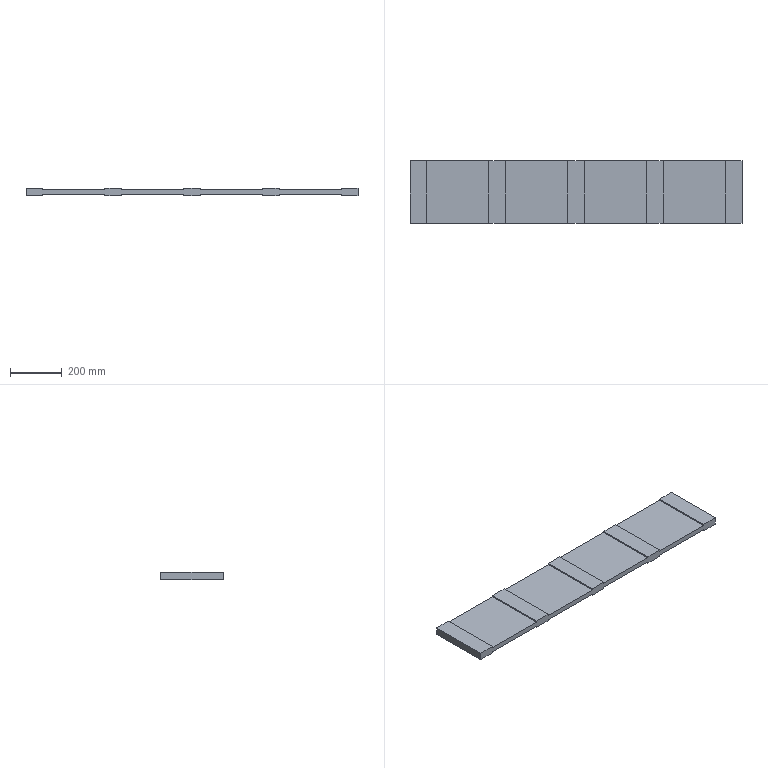Part | SolidWorks | features Extrusion 1, ICE 1 | 1 solid | 38 faces | box 1280 x 240 x 30 mm | volume 6912000 mm3 | plane 38
STEP:
#1=CARTESIAN_POINT('',(672.,0.,20.));
#2=VERTEX_POINT('',#1);
#3=CARTESIAN_POINT('',(912.,0.,20.));
#4=VERTEX_POINT('',#3);
#5=CARTESIAN_POINT('',(0.,0.,20.));
#6=DIRECTION('',(1.,0.,0.));
#7=VECTOR('',#6,1000.);
#8=LINE('',#5,#7);
#9=EDGE_CURVE('',#2,#4,#8,.T.);
#10=ORIENTED_EDGE('',*,*,#9,.T.);
#11=CARTESIAN_POINT('',(912.,240.,20.));
#12=VERTEX_POINT('',#11);
#13=CARTESIAN_POINT('',(912.,0.,20.));
#14=DIRECTION('',(0.,1.,0.));
#15=VECTOR('',#14,1000.);
#16=LINE('',#13,#15);
#17=EDGE_CURVE('',#4,#12,#16,.T.);
#18=ORIENTED_EDGE('',*,*,#17,.T.);
#19=CARTESIAN_POINT('',(672.,240.,20.));
#20=VERTEX_POINT('',#19);
#21=CARTESIAN_POINT('',(0.,240.,20.));
#22=DIRECTION('',(-1.,0.,0.));
#23=VECTOR('',#22,1000.);
#24=LINE('',#21,#23);
#25=EDGE_CURVE('',#12,#20,#24,.T.);
#26=ORIENTED_EDGE('',*,*,#25,.T.);
#27=CARTESIAN_POINT('',(672.,0.,20.));
#28=DIRECTION('',(0.,-1.,0.));
#29=VECTOR('',#28,1000.);
#30=LINE('',#27,#29);
#31=EDGE_CURVE('',#20,#2,#30,.T.);
#32=ORIENTED_EDGE('',*,*,#31,.T.);
#33=EDGE_LOOP('',(#10,#18,#26,#32));
#34=FACE_OUTER_BOUND('',#33,.T.);
#35=CARTESIAN_POINT('',(0.,0.,20.));
#36=DIRECTION('',(0.,0.,-1.));
#37=DIRECTION('',(-1.,0.,0.));
#38=AXIS2_PLACEMENT_3D('',#35,#36,#37);
#39=PLANE('',#38);
#40=ADVANCED_FACE('',(#34),#39,.F.);
#41=CARTESIAN_POINT('',(912.,0.,0.));
#42=VERTEX_POINT('',#41);
#43=CARTESIAN_POINT('',(912.,240.,0.));
#44=VERTEX_POINT('',#43);
#45=CARTESIAN_POINT('',(912.,0.,0.));
#46=DIRECTION('',(0.,1.,0.));
#47=VECTOR('',#46,1000.);
#48=LINE('',#45,#47);
#49=EDGE_CURVE('',#42,#44,#48,.T.);
#50=ORIENTED_EDGE('',*,*,#49,.F.);
#51=CARTESIAN_POINT('',(672.,0.,0.));
#52=VERTEX_POINT('',#51);
#53=CARTESIAN_POINT('',(0.,0.,0.));
#54=DIRECTION('',(1.,0.,0.));
#55=VECTOR('',#54,1000.);
#56=LINE('',#53,#55);
#57=EDGE_CURVE('',#52,#42,#56,.T.);
#58=ORIENTED_EDGE('',*,*,#57,.F.);
#59=CARTESIAN_POINT('',(672.,240.,0.));
#60=VERTEX_POINT('',#59);
#61=CARTESIAN_POINT('',(672.,0.,0.));
#62=DIRECTION('',(0.,-1.,0.));
#63=VECTOR('',#62,1000.);
#64=LINE('',#61,#63);
#65=EDGE_CURVE('',#60,#52,#64,.T.);
#66=ORIENTED_EDGE('',*,*,#65,.F.);
#67=CARTESIAN_POINT('',(0.,240.,0.));
#68=DIRECTION('',(-1.,0.,0.));
#69=VECTOR('',#68,1000.);
#70=LINE('',#67,#69);
#71=EDGE_CURVE('',#44,#60,#70,.T.);
#72=ORIENTED_EDGE('',*,*,#71,.F.);
#73=EDGE_LOOP('',(#50,#58,#66,#72));
#74=FACE_OUTER_BOUND('',#73,.T.);
#75=CARTESIAN_POINT('',(0.,0.,0.));
#76=DIRECTION('',(0.,0.,-1.));
#77=DIRECTION('',(-1.,0.,0.));
#78=AXIS2_PLACEMENT_3D('',#75,#76,#77);
#79=PLANE('',#78);
#80=ADVANCED_FACE('',(#74),#79,.T.);
#81=CARTESIAN_POINT('',(368.,0.,20.));
#82=VERTEX_POINT('',#81);
#83=CARTESIAN_POINT('',(608.,0.,20.));
#84=VERTEX_POINT('',#83);
#85=CARTESIAN_POINT('',(0.,0.,20.));
#86=DIRECTION('',(1.,0.,0.));
#87=VECTOR('',#86,1000.);
#88=LINE('',#85,#87);
#89=EDGE_CURVE('',#82,#84,#88,.T.);
#90=ORIENTED_EDGE('',*,*,#89,.T.);
#91=CARTESIAN_POINT('',(608.,240.,20.));
#92=VERTEX_POINT('',#91);
#93=CARTESIAN_POINT('',(608.,0.,20.));
#94=DIRECTION('',(0.,1.,0.));
#95=VECTOR('',#94,1000.);
#96=LINE('',#93,#95);
#97=EDGE_CURVE('',#84,#92,#96,.T.);
#98=ORIENTED_EDGE('',*,*,#97,.T.);
#99=CARTESIAN_POINT('',(368.,240.,20.));
#100=VERTEX_POINT('',#99);
#101=CARTESIAN_POINT('',(0.,240.,20.));
#102=DIRECTION('',(-1.,0.,0.));
#103=VECTOR('',#102,1000.);
#104=LINE('',#101,#103);
#105=EDGE_CURVE('',#92,#100,#104,.T.);
#106=ORIENTED_EDGE('',*,*,#105,.T.);
#107=CARTESIAN_POINT('',(368.,0.,20.));
#108=DIRECTION('',(0.,-1.,0.));
#109=VECTOR('',#108,1000.);
#110=LINE('',#107,#109);
#111=EDGE_CURVE('',#100,#82,#110,.T.);
#112=ORIENTED_EDGE('',*,*,#111,.T.);
#113=EDGE_LOOP('',(#90,#98,#106,#112));
#114=FACE_OUTER_BOUND('',#113,.T.);
#115=CARTESIAN_POINT('',(0.,0.,20.));
#116=DIRECTION('',(0.,0.,-1.));
#117=DIRECTION('',(-1.,0.,0.));
#118=AXIS2_PLACEMENT_3D('',#115,#116,#117);
#119=PLANE('',#118);
#120=ADVANCED_FACE('',(#114),#119,.F.);
#121=CARTESIAN_POINT('',(608.,0.,0.));
#122=VERTEX_POINT('',#121);
#123=CARTESIAN_POINT('',(608.,240.,0.));
#124=VERTEX_POINT('',#123);
#125=CARTESIAN_POINT('',(608.,0.,0.));
#126=DIRECTION('',(0.,1.,0.));
#127=VECTOR('',#126,1000.);
#128=LINE('',#125,#127);
#129=EDGE_CURVE('',#122,#124,#128,.T.);
#130=ORIENTED_EDGE('',*,*,#129,.F.);
#131=CARTESIAN_POINT('',(368.,0.,0.));
#132=VERTEX_POINT('',#131);
#133=CARTESIAN_POINT('',(0.,0.,0.));
#134=DIRECTION('',(1.,0.,0.));
#135=VECTOR('',#134,1000.);
#136=LINE('',#133,#135);
#137=EDGE_CURVE('',#132,#122,#136,.T.);
#138=ORIENTED_EDGE('',*,*,#137,.F.);
#139=CARTESIAN_POINT('',(368.,240.,0.));
#140=VERTEX_POINT('',#139);
#141=CARTESIAN_POINT('',(368.,0.,0.));
#142=DIRECTION('',(0.,-1.,0.));
#143=VECTOR('',#142,1000.);
#144=LINE('',#141,#143);
#145=EDGE_CURVE('',#140,#132,#144,.T.);
#146=ORIENTED_EDGE('',*,*,#145,.F.);
#147=CARTESIAN_POINT('',(0.,240.,0.));
#148=DIRECTION('',(-1.,0.,0.));
#149=VECTOR('',#148,1000.);
#150=LINE('',#147,#149);
#151=EDGE_CURVE('',#124,#140,#150,.T.);
#152=ORIENTED_EDGE('',*,*,#151,.F.);
#153=EDGE_LOOP('',(#130,#138,#146,#152));
#154=FACE_OUTER_BOUND('',#153,.T.);
#155=CARTESIAN_POINT('',(0.,0.,0.));
#156=DIRECTION('',(0.,0.,-1.));
#157=DIRECTION('',(-1.,0.,0.));
#158=AXIS2_PLACEMENT_3D('',#155,#156,#157);
#159=PLANE('',#158);
#160=ADVANCED_FACE('',(#154),#159,.T.);
#161=CARTESIAN_POINT('',(64.,0.,20.));
#162=VERTEX_POINT('',#161);
#163=CARTESIAN_POINT('',(304.,0.,20.));
#164=VERTEX_POINT('',#163);
#165=CARTESIAN_POINT('',(0.,0.,20.));
#166=DIRECTION('',(1.,0.,0.));
#167=VECTOR('',#166,1000.);
#168=LINE('',#165,#167);
#169=EDGE_CURVE('',#162,#164,#168,.T.);
#170=ORIENTED_EDGE('',*,*,#169,.T.);
#171=CARTESIAN_POINT('',(304.,240.,20.));
#172=VERTEX_POINT('',#171);
#173=CARTESIAN_POINT('',(304.,0.,20.));
#174=DIRECTION('',(0.,1.,0.));
#175=VECTOR('',#174,1000.);
#176=LINE('',#173,#175);
#177=EDGE_CURVE('',#164,#172,#176,.T.);
#178=ORIENTED_EDGE('',*,*,#177,.T.);
#179=CARTESIAN_POINT('',(64.,240.,20.));
#180=VERTEX_POINT('',#179);
#181=CARTESIAN_POINT('',(0.,240.,20.));
#182=DIRECTION('',(-1.,0.,0.));
#183=VECTOR('',#182,1000.);
#184=LINE('',#181,#183);
#185=EDGE_CURVE('',#172,#180,#184,.T.);
#186=ORIENTED_EDGE('',*,*,#185,.T.);
#187=CARTESIAN_POINT('',(64.,0.,20.));
#188=DIRECTION('',(0.,-1.,0.));
#189=VECTOR('',#188,1000.);
#190=LINE('',#187,#189);
#191=EDGE_CURVE('',#180,#162,#190,.T.);
#192=ORIENTED_EDGE('',*,*,#191,.T.);
#193=EDGE_LOOP('',(#170,#178,#186,#192));
#194=FACE_OUTER_BOUND('',#193,.T.);
#195=CARTESIAN_POINT('',(0.,0.,20.));
#196=DIRECTION('',(0.,0.,-1.));
#197=DIRECTION('',(-1.,0.,0.));
#198=AXIS2_PLACEMENT_3D('',#195,#196,#197);
#199=PLANE('',#198);
#200=ADVANCED_FACE('',(#194),#199,.F.);
#201=CARTESIAN_POINT('',(304.,0.,0.));
#202=VERTEX_POINT('',#201);
#203=CARTESIAN_POINT('',(304.,240.,0.));
#204=VERTEX_POINT('',#203);
#205=CARTESIAN_POINT('',(304.,0.,0.));
#206=DIRECTION('',(0.,1.,0.));
#207=VECTOR('',#206,1000.);
#208=LINE('',#205,#207);
#209=EDGE_CURVE('',#202,#204,#208,.T.);
#210=ORIENTED_EDGE('',*,*,#209,.F.);
#211=CARTESIAN_POINT('',(64.,0.,0.));
#212=VERTEX_POINT('',#211);
#213=CARTESIAN_POINT('',(0.,0.,0.));
#214=DIRECTION('',(1.,0.,0.));
#215=VECTOR('',#214,1000.);
#216=LINE('',#213,#215);
#217=EDGE_CURVE('',#212,#202,#216,.T.);
#218=ORIENTED_EDGE('',*,*,#217,.F.);
#219=CARTESIAN_POINT('',(64.,240.,0.));
#220=VERTEX_POINT('',#219);
#221=CARTESIAN_POINT('',(64.,0.,0.));
#222=DIRECTION('',(0.,-1.,0.));
#223=VECTOR('',#222,1000.);
#224=LINE('',#221,#223);
#225=EDGE_CURVE('',#220,#212,#224,.T.);
#226=ORIENTED_EDGE('',*,*,#225,.F.);
#227=CARTESIAN_POINT('',(0.,240.,0.));
#228=DIRECTION('',(-1.,0.,0.));
#229=VECTOR('',#228,1000.);
#230=LINE('',#227,#229);
#231=EDGE_CURVE('',#204,#220,#230,.T.);
#232=ORIENTED_EDGE('',*,*,#231,.F.);
#233=EDGE_LOOP('',(#210,#218,#226,#232));
#234=FACE_OUTER_BOUND('',#233,.T.);
#235=CARTESIAN_POINT('',(0.,0.,0.));
#236=DIRECTION('',(0.,0.,-1.));
#237=DIRECTION('',(-1.,0.,0.));
#238=AXIS2_PLACEMENT_3D('',#235,#236,#237);
#239=PLANE('',#238);
#240=ADVANCED_FACE('',(#234),#239,.T.);
#241=CARTESIAN_POINT('',(0.,240.,25.));
#242=VERTEX_POINT('',#241);
#243=CARTESIAN_POINT('',(0.,240.,-5.));
#244=VERTEX_POINT('',#243);
#245=CARTESIAN_POINT('',(0.,240.,20.));
#246=DIRECTION('',(0.,0.,-1.));
#247=VECTOR('',#246,1000.);
#248=LINE('',#245,#247);
#249=EDGE_CURVE('',#242,#244,#248,.T.);
#250=ORIENTED_EDGE('',*,*,#249,.T.);
#251=CARTESIAN_POINT('',(0.,0.,-5.));
#252=VERTEX_POINT('',#251);
#253=CARTESIAN_POINT('',(0.,240.,-5.));
#254=DIRECTION('',(0.,-1.,0.));
#255=VECTOR('',#254,1000.);
#256=LINE('',#253,#255);
#257=EDGE_CURVE('',#244,#252,#256,.T.);
#258=ORIENTED_EDGE('',*,*,#257,.T.);
#259=CARTESIAN_POINT('',(0.,0.,25.));
#260=VERTEX_POINT('',#259);
#261=CARTESIAN_POINT('',(0.,0.,20.));
#262=DIRECTION('',(0.,0.,-1.));
#263=VECTOR('',#262,1000.);
#264=LINE('',#261,#263);
#265=EDGE_CURVE('',#260,#252,#264,.T.);
#266=ORIENTED_EDGE('',*,*,#265,.F.);
#267=CARTESIAN_POINT('',(0.,240.,25.));
#268=DIRECTION('',(0.,-1.,0.));
#269=VECTOR('',#268,1000.);
#270=LINE('',#267,#269);
#271=EDGE_CURVE('',#242,#260,#270,.T.);
#272=ORIENTED_EDGE('',*,*,#271,.F.);
#273=EDGE_LOOP('',(#250,#258,#266,#272));
#274=FACE_OUTER_BOUND('',#273,.T.);
#275=CARTESIAN_POINT('',(0.,0.,20.));
#276=DIRECTION('',(1.,0.,0.));
#277=DIRECTION('',(0.,0.,-1.));
#278=AXIS2_PLACEMENT_3D('',#275,#276,#277);
#279=PLANE('',#278);
#280=ADVANCED_FACE('',(#274),#279,.F.);
#281=CARTESIAN_POINT('',(976.,0.,0.));
#282=VERTEX_POINT('',#281);
#283=CARTESIAN_POINT('',(1216.,0.,0.));
#284=VERTEX_POINT('',#283);
#285=CARTESIAN_POINT('',(0.,0.,0.));
#286=DIRECTION('',(1.,0.,0.));
#287=VECTOR('',#286,1000.);
#288=LINE('',#285,#287);
#289=EDGE_CURVE('',#282,#284,#288,.T.);
#290=ORIENTED_EDGE('',*,*,#289,.T.);
#291=CARTESIAN_POINT('',(1216.,0.,-5.));
#292=VERTEX_POINT('',#291);
#293=CARTESIAN_POINT('',(1216.,0.,25.));
#294=DIRECTION('',(0.,0.,-1.));
#295=VECTOR('',#294,1000.);
#296=LINE('',#293,#295);
#297=EDGE_CURVE('',#284,#292,#296,.T.);
#298=ORIENTED_EDGE('',*,*,#297,.T.);
#299=CARTESIAN_POINT('',(1280.,0.,-5.));
#300=VERTEX_POINT('',#299);
#301=CARTESIAN_POINT('',(1216.,0.,-5.));
#302=DIRECTION('',(1.,0.,0.));
#303=VECTOR('',#302,1000.);
#304=LINE('',#301,#303);
#305=EDGE_CURVE('',#292,#300,#304,.T.);
#306=ORIENTED_EDGE('',*,*,#305,.T.);
#307=CARTESIAN_POINT('',(1280.,0.,25.));
#308=VERTEX_POINT('',#307);
#309=CARTESIAN_POINT('',(1280.,0.,25.));
#310=DIRECTION('',(0.,0.,1.));
#311=VECTOR('',#310,1000.);
#312=LINE('',#309,#311);
#313=EDGE_CURVE('',#300,#308,#312,.T.);
#314=ORIENTED_EDGE('',*,*,#313,.T.);
#315=CARTESIAN_POINT('',(1216.,0.,25.));
#316=VERTEX_POINT('',#315);
#317=CARTESIAN_POINT('',(1216.,0.,25.));
#318=DIRECTION('',(-1.,0.,0.));
#319=VECTOR('',#318,1000.);
#320=LINE('',#317,#319);
#321=EDGE_CURVE('',#308,#316,#320,.T.);
#322=ORIENTED_EDGE('',*,*,#321,.T.);
#323=CARTESIAN_POINT('',(1216.,0.,20.));
#324=VERTEX_POINT('',#323);
#325=CARTESIAN_POINT('',(1216.,0.,25.));
#326=DIRECTION('',(0.,0.,-1.));
#327=VECTOR('',#326,1000.);
#328=LINE('',#325,#327);
#329=EDGE_CURVE('',#316,#324,#328,.T.);
#330=ORIENTED_EDGE('',*,*,#329,.T.);
#331=CARTESIAN_POINT('',(976.,0.,20.));
#332=VERTEX_POINT('',#331);
#333=CARTESIAN_POINT('',(0.,0.,20.));
#334=DIRECTION('',(1.,0.,0.));
#335=VECTOR('',#334,1000.);
#336=LINE('',#333,#335);
#337=EDGE_CURVE('',#332,#324,#336,.T.);
#338=ORIENTED_EDGE('',*,*,#337,.F.);
#339=CARTESIAN_POINT('',(976.,0.,25.));
#340=VERTEX_POINT('',#339);
#341=CARTESIAN_POINT('',(976.,0.,25.));
#342=DIRECTION('',(0.,0.,1.));
#343=VECTOR('',#342,1000.);
#344=LINE('',#341,#343);
#345=EDGE_CURVE('',#332,#340,#344,.T.);
#346=ORIENTED_EDGE('',*,*,#345,.T.);
#347=CARTESIAN_POINT('',(912.,0.,25.));
#348=VERTEX_POINT('',#347);
#349=CARTESIAN_POINT('',(912.,0.,25.));
#350=DIRECTION('',(-1.,0.,0.));
#351=VECTOR('',#350,1000.);
#352=LINE('',#349,#351);
#353=EDGE_CURVE('',#340,#348,#352,.T.);
#354=ORIENTED_EDGE('',*,*,#353,.T.);
#355=CARTESIAN_POINT('',(912.,0.,25.));
#356=DIRECTION('',(0.,0.,-1.));
#357=VECTOR('',#356,1000.);
#358=LINE('',#355,#357);
#359=EDGE_CURVE('',#348,#4,#358,.T.);
#360=ORIENTED_EDGE('',*,*,#359,.T.);
#361=ORIENTED_EDGE('',*,*,#9,.F.);
#362=CARTESIAN_POINT('',(672.,0.,25.));
#363=VERTEX_POINT('',#362);
#364=CARTESIAN_POINT('',(672.,0.,25.));
#365=DIRECTION('',(0.,0.,1.));
#366=VECTOR('',#365,1000.);
#367=LINE('',#364,#366);
#368=EDGE_CURVE('',#2,#363,#367,.T.);
#369=ORIENTED_EDGE('',*,*,#368,.T.);
#370=CARTESIAN_POINT('',(608.,0.,25.));
#371=VERTEX_POINT('',#370);
#372=CARTESIAN_POINT('',(608.,0.,25.));
#373=DIRECTION('',(-1.,0.,0.));
#374=VECTOR('',#373,1000.);
#375=LINE('',#372,#374);
#376=EDGE_CURVE('',#363,#371,#375,.T.);
#377=ORIENTED_EDGE('',*,*,#376,.T.);
#378=CARTESIAN_POINT('',(608.,0.,25.));
#379=DIRECTION('',(0.,0.,-1.));
#380=VECTOR('',#379,1000.);
#381=LINE('',#378,#380);
#382=EDGE_CURVE('',#371,#84,#381,.T.);
#383=ORIENTED_EDGE('',*,*,#382,.T.);
#384=ORIENTED_EDGE('',*,*,#89,.F.);
#385=CARTESIAN_POINT('',(368.,0.,25.));
#386=VERTEX_POINT('',#385);
#387=CARTESIAN_POINT('',(368.,0.,25.));
#388=DIRECTION('',(0.,0.,1.));
#389=VECTOR('',#388,1000.);
#390=LINE('',#387,#389);
#391=EDGE_CURVE('',#82,#386,#390,.T.);
#392=ORIENTED_EDGE('',*,*,#391,.T.);
#393=CARTESIAN_POINT('',(304.,0.,25.));
#394=VERTEX_POINT('',#393);
#395=CARTESIAN_POINT('',(304.,0.,25.));
#396=DIRECTION('',(-1.,0.,0.));
#397=VECTOR('',#396,1000.);
#398=LINE('',#395,#397);
#399=EDGE_CURVE('',#386,#394,#398,.T.);
#400=ORIENTED_EDGE('',*,*,#399,.T.);
#401=CARTESIAN_POINT('',(304.,0.,25.));
#402=DIRECTION('',(0.,0.,-1.));
#403=VECTOR('',#402,1000.);
#404=LINE('',#401,#403);
#405=EDGE_CURVE('',#394,#164,#404,.T.);
#406=ORIENTED_EDGE('',*,*,#405,.T.);
#407=ORIENTED_EDGE('',*,*,#169,.F.);
#408=CARTESIAN_POINT('',(64.,0.,25.));
#409=VERTEX_POINT('',#408);
#410=CARTESIAN_POINT('',(64.,0.,-5.));
#411=DIRECTION('',(0.,0.,1.));
#412=VECTOR('',#411,1000.);
#413=LINE('',#410,#412);
#414=EDGE_CURVE('',#162,#409,#413,.T.);
#415=ORIENTED_EDGE('',*,*,#414,.T.);
#416=CARTESIAN_POINT('',(0.,0.,25.));
#417=DIRECTION('',(-1.,0.,0.));
#418=VECTOR('',#417,1000.);
#419=LINE('',#416,#418);
#420=EDGE_CURVE('',#409,#260,#419,.T.);
#421=ORIENTED_EDGE('',*,*,#420,.T.);
#422=ORIENTED_EDGE('',*,*,#265,.T.);
#423=CARTESIAN_POINT('',(64.,0.,-5.));
#424=VERTEX_POINT('',#423);
#425=CARTESIAN_POINT('',(0.,0.,-5.));
#426=DIRECTION('',(1.,0.,0.));
#427=VECTOR('',#426,1000.);
#428=LINE('',#425,#427);
#429=EDGE_CURVE('',#252,#424,#428,.T.);
#430=ORIENTED_EDGE('',*,*,#429,.T.);
#431=CARTESIAN_POINT('',(64.,0.,-5.));
#432=DIRECTION('',(0.,0.,1.));
#433=VECTOR('',#432,1000.);
#434=LINE('',#431,#433);
#435=EDGE_CURVE('',#424,#212,#434,.T.);
#436=ORIENTED_EDGE('',*,*,#435,.T.);
#437=ORIENTED_EDGE('',*,*,#217,.T.);
#438=CARTESIAN_POINT('',(304.,0.,-5.));
#439=VERTEX_POINT('',#438);
#440=CARTESIAN_POINT('',(304.,0.,25.));
#441=DIRECTION('',(0.,0.,-1.));
#442=VECTOR('',#441,1000.);
#443=LINE('',#440,#442);
#444=EDGE_CURVE('',#202,#439,#443,.T.);
#445=ORIENTED_EDGE('',*,*,#444,.T.);
#446=CARTESIAN_POINT('',(368.,0.,-5.));
#447=VERTEX_POINT('',#446);
#448=CARTESIAN_POINT('',(304.,0.,-5.));
#449=DIRECTION('',(1.,0.,0.));
#450=VECTOR('',#449,1000.);
#451=LINE('',#448,#450);
#452=EDGE_CURVE('',#439,#447,#451,.T.);
#453=ORIENTED_EDGE('',*,*,#452,.T.);
#454=CARTESIAN_POINT('',(368.,0.,25.));
#455=DIRECTION('',(0.,0.,1.));
#456=VECTOR('',#455,1000.);
#457=LINE('',#454,#456);
#458=EDGE_CURVE('',#447,#132,#457,.T.);
#459=ORIENTED_EDGE('',*,*,#458,.T.);
#460=ORIENTED_EDGE('',*,*,#137,.T.);
#461=CARTESIAN_POINT('',(608.,0.,-5.));
#462=VERTEX_POINT('',#461);
#463=CARTESIAN_POINT('',(608.,0.,25.));
#464=DIRECTION('',(0.,0.,-1.));
#465=VECTOR('',#464,1000.);
#466=LINE('',#463,#465);
#467=EDGE_CURVE('',#122,#462,#466,.T.);
#468=ORIENTED_EDGE('',*,*,#467,.T.);
#469=CARTESIAN_POINT('',(672.,0.,-5.));
#470=VERTEX_POINT('',#469);
#471=CARTESIAN_POINT('',(608.,0.,-5.));
#472=DIRECTION('',(1.,0.,0.));
#473=VECTOR('',#472,1000.);
#474=LINE('',#471,#473);
#475=EDGE_CURVE('',#462,#470,#474,.T.);
#476=ORIENTED_EDGE('',*,*,#475,.T.);
#477=CARTESIAN_POINT('',(672.,0.,25.));
#478=DIRECTION('',(0.,0.,1.));
#479=VECTOR('',#478,1000.);
#480=LINE('',#477,#479);
#481=EDGE_CURVE('',#470,#52,#480,.T.);
#482=ORIENTED_EDGE('',*,*,#481,.T.);
#483=ORIENTED_EDGE('',*,*,#57,.T.);
#484=CARTESIAN_POINT('',(912.,0.,-5.));
#485=VERTEX_POINT('',#484);
#486=CARTESIAN_POINT('',(912.,0.,25.));
#487=DIRECTION('',(0.,0.,-1.));
#488=VECTOR('',#487,1000.);
#489=LINE('',#486,#488);
#490=EDGE_CURVE('',#42,#485,#489,.T.);
#491=ORIENTED_EDGE('',*,*,#490,.T.);
#492=CARTESIAN_POINT('',(976.,0.,-5.));
#493=VERTEX_POINT('',#492);
#494=CARTESIAN_POINT('',(912.,0.,-5.));
#495=DIRECTION('',(1.,0.,0.));
#496=VECTOR('',#495,1000.);
#497=LINE('',#494,#496);
#498=EDGE_CURVE('',#485,#493,#497,.T.);
#499=ORIENTED_EDGE('',*,*,#498,.T.);
#500=CARTESIAN_POINT('',(976.,0.,25.));
#501=DIRECTION('',(0.,0.,1.));
#502=VECTOR('',#501,1000.);
#503=LINE('',#500,#502);
#504=EDGE_CURVE('',#493,#282,#503,.T.);
#505=ORIENTED_EDGE('',*,*,#504,.T.);
#506=EDGE_LOOP('',(#290,#298,#306,#314,#322,#330,#338,#346,#354,#360,#361,#369,#377,#383,#384,#392,#400,#406,#407,#415,#421,#422,#430,#436,#437,#445,#453,#459,#460,#468,#476,#482,#483,#491,#499,#505));
#507=FACE_OUTER_BOUND('',#506,.T.);
#508=CARTESIAN_POINT('',(0.,0.,20.));
#509=DIRECTION('',(0.,1.,0.));
#510=DIRECTION('',(0.,0.,1.));
#511=AXIS2_PLACEMENT_3D('',#508,#509,#510);
#512=PLANE('',#511);
#513=ADVANCED_FACE('',(#507),#512,.F.);
#514=CARTESIAN_POINT('',(1216.,240.,20.));
#515=VERTEX_POINT('',#514);
#516=CARTESIAN_POINT('',(976.,240.,20.));
#517=VERTEX_POINT('',#516);
#518=CARTESIAN_POINT('',(0.,240.,20.));
#519=DIRECTION('',(-1.,0.,0.));
#520=VECTOR('',#519,1000.);
#521=LINE('',#518,#520);
#522=EDGE_CURVE('',#515,#517,#521,.T.);
#523=ORIENTED_EDGE('',*,*,#522,.F.);
#524=CARTESIAN_POINT('',(1216.,240.,25.));
#525=VERTEX_POINT('',#524);
#526=CARTESIAN_POINT('',(1216.,240.,25.));
#527=DIRECTION('',(0.,0.,-1.));
#528=VECTOR('',#527,1000.);
#529=LINE('',#526,#528);
#530=EDGE_CURVE('',#525,#515,#529,.T.);
#531=ORIENTED_EDGE('',*,*,#530,.F.);
#532=CARTESIAN_POINT('',(1280.,240.,25.));
#533=VERTEX_POINT('',#532);
#534=CARTESIAN_POINT('',(1216.,240.,25.));
#535=DIRECTION('',(-1.,0.,0.));
#536=VECTOR('',#535,1000.);
#537=LINE('',#534,#536);
#538=EDGE_CURVE('',#533,#525,#537,.T.);
#539=ORIENTED_EDGE('',*,*,#538,.F.);
#540=CARTESIAN_POINT('',(1280.,240.,-5.));
#541=VERTEX_POINT('',#540);
#542=CARTESIAN_POINT('',(1280.,240.,25.));
#543=DIRECTION('',(0.,0.,1.));
#544=VECTOR('',#543,1000.);
#545=LINE('',#542,#544);
#546=EDGE_CURVE('',#541,#533,#545,.T.);
#547=ORIENTED_EDGE('',*,*,#546,.F.);
#548=CARTESIAN_POINT('',(1216.,240.,-5.));
#549=VERTEX_POINT('',#548);
#550=CARTESIAN_POINT('',(1216.,240.,-5.));
#551=DIRECTION('',(1.,0.,0.));
#552=VECTOR('',#551,1000.);
#553=LINE('',#550,#552);
#554=EDGE_CURVE('',#549,#541,#553,.T.);
#555=ORIENTED_EDGE('',*,*,#554,.F.);
#556=CARTESIAN_POINT('',(1216.,240.,0.));
#557=VERTEX_POINT('',#556);
#558=CARTESIAN_POINT('',(1216.,240.,25.));
#559=DIRECTION('',(0.,0.,-1.));
#560=VECTOR('',#559,1000.);
#561=LINE('',#558,#560);
#562=EDGE_CURVE('',#557,#549,#561,.T.);
#563=ORIENTED_EDGE('',*,*,#562,.F.);
#564=CARTESIAN_POINT('',(976.,240.,0.));
#565=VERTEX_POINT('',#564);
#566=CARTESIAN_POINT('',(0.,240.,0.));
#567=DIRECTION('',(-1.,0.,0.));
#568=VECTOR('',#567,1000.);
#569=LINE('',#566,#568);
#570=EDGE_CURVE('',#557,#565,#569,.T.);
#571=ORIENTED_EDGE('',*,*,#570,.T.);
#572=CARTESIAN_POINT('',(976.,240.,-5.));
#573=VERTEX_POINT('',#572);
#574=CARTESIAN_POINT('',(976.,240.,25.));
#575=DIRECTION('',(0.,0.,1.));
#576=VECTOR('',#575,1000.);
#577=LINE('',#574,#576);
#578=EDGE_CURVE('',#573,#565,#577,.T.);
#579=ORIENTED_EDGE('',*,*,#578,.F.);
#580=CARTESIAN_POINT('',(912.,240.,-5.));
#581=VERTEX_POINT('',#580);
#582=CARTESIAN_POINT('',(912.,240.,-5.));
#583=DIRECTION('',(1.,0.,0.));
#584=VECTOR('',#583,1000.);
#585=LINE('',#582,#584);
#586=EDGE_CURVE('',#581,#573,#585,.T.);
#587=ORIENTED_EDGE('',*,*,#586,.F.);
#588=CARTESIAN_POINT('',(912.,240.,25.));
#589=DIRECTION('',(0.,0.,-1.));
#590=VECTOR('',#589,1000.);
#591=LINE('',#588,#590);
#592=EDGE_CURVE('',#44,#581,#591,.T.);
#593=ORIENTED_EDGE('',*,*,#592,.F.);
#594=ORIENTED_EDGE('',*,*,#71,.T.);
#595=CARTESIAN_POINT('',(672.,240.,-5.));
#596=VERTEX_POINT('',#595);
#597=CARTESIAN_POINT('',(672.,240.,25.));
#598=DIRECTION('',(0.,0.,1.));
#599=VECTOR('',#598,1000.);
#600=LINE('',#597,#599);
#601=EDGE_CURVE('',#596,#60,#600,.T.);
#602=ORIENTED_EDGE('',*,*,#601,.F.);
#603=CARTESIAN_POINT('',(608.,240.,-5.));
#604=VERTEX_POINT('',#603);
#605=CARTESIAN_POINT('',(608.,240.,-5.));
#606=DIRECTION('',(1.,0.,0.));
#607=VECTOR('',#606,1000.);
#608=LINE('',#605,#607);
#609=EDGE_CURVE('',#604,#596,#608,.T.);
#610=ORIENTED_EDGE('',*,*,#609,.F.);
#611=CARTESIAN_POINT('',(608.,240.,25.));
#612=DIRECTION('',(0.,0.,-1.));
#613=VECTOR('',#612,1000.);
#614=LINE('',#611,#613);
#615=EDGE_CURVE('',#124,#604,#614,.T.);
#616=ORIENTED_EDGE('',*,*,#615,.F.);
#617=ORIENTED_EDGE('',*,*,#151,.T.);
#618=CARTESIAN_POINT('',(368.,240.,-5.));
#619=VERTEX_POINT('',#618);
#620=CARTESIAN_POINT('',(368.,240.,25.));
#621=DIRECTION('',(0.,0.,1.));
#622=VECTOR('',#621,1000.);
#623=LINE('',#620,#622);
#624=EDGE_CURVE('',#619,#140,#623,.T.);
#625=ORIENTED_EDGE('',*,*,#624,.F.);
#626=CARTESIAN_POINT('',(304.,240.,-5.));
#627=VERTEX_POINT('',#626);
#628=CARTESIAN_POINT('',(304.,240.,-5.));
#629=DIRECTION('',(1.,0.,0.));
#630=VECTOR('',#629,1000.);
#631=LINE('',#628,#630);
#632=EDGE_CURVE('',#627,#619,#631,.T.);
#633=ORIENTED_EDGE('',*,*,#632,.F.);
#634=CARTESIAN_POINT('',(304.,240.,25.));
#635=DIRECTION('',(0.,0.,-1.));
#636=VECTOR('',#635,1000.);
#637=LINE('',#634,#636);
#638=EDGE_CURVE('',#204,#627,#637,.T.);
#639=ORIENTED_EDGE('',*,*,#638,.F.);
#640=ORIENTED_EDGE('',*,*,#231,.T.);
#641=CARTESIAN_POINT('',(64.,240.,-5.));
#642=VERTEX_POINT('',#641);
#643=CARTESIAN_POINT('',(64.,240.,-5.));
#644=DIRECTION('',(0.,0.,1.));
#645=VECTOR('',#644,1000.);
#646=LINE('',#643,#645);
#647=EDGE_CURVE('',#642,#220,#646,.T.);
#648=ORIENTED_EDGE('',*,*,#647,.F.);
#649=CARTESIAN_POINT('',(0.,240.,-5.));
#650=DIRECTION('',(1.,0.,0.));
#651=VECTOR('',#650,1000.);
#652=LINE('',#649,#651);
#653=EDGE_CURVE('',#244,#642,#652,.T.);
#654=ORIENTED_EDGE('',*,*,#653,.F.);
#655=ORIENTED_EDGE('',*,*,#249,.F.);
#656=CARTESIAN_POINT('',(64.,240.,25.));
#657=VERTEX_POINT('',#656);
#658=CARTESIAN_POINT('',(0.,240.,25.));
#659=DIRECTION('',(-1.,0.,0.));
#660=VECTOR('',#659,1000.);
#661=LINE('',#658,#660);
#662=EDGE_CURVE('',#657,#242,#661,.T.);
#663=ORIENTED_EDGE('',*,*,#662,.F.);
#664=CARTESIAN_POINT('',(64.,240.,-5.));
#665=DIRECTION('',(0.,0.,1.));
#666=VECTOR('',#665,1000.);
#667=LINE('',#664,#666);
#668=EDGE_CURVE('',#180,#657,#667,.T.);
#669=ORIENTED_EDGE('',*,*,#668,.F.);
#670=ORIENTED_EDGE('',*,*,#185,.F.);
#671=CARTESIAN_POINT('',(304.,240.,25.));
#672=VERTEX_POINT('',#671);
#673=CARTESIAN_POINT('',(304.,240.,25.));
#674=DIRECTION('',(0.,0.,-1.));
#675=VECTOR('',#674,1000.);
#676=LINE('',#673,#675);
#677=EDGE_CURVE('',#672,#172,#676,.T.);
#678=ORIENTED_EDGE('',*,*,#677,.F.);
#679=CARTESIAN_POINT('',(368.,240.,25.));
#680=VERTEX_POINT('',#679);
#681=CARTESIAN_POINT('',(304.,240.,25.));
#682=DIRECTION('',(-1.,0.,0.));
#683=VECTOR('',#682,1000.);
#684=LINE('',#681,#683);
#685=EDGE_CURVE('',#680,#672,#684,.T.);
#686=ORIENTED_EDGE('',*,*,#685,.F.);
#687=CARTESIAN_POINT('',(368.,240.,25.));
#688=DIRECTION('',(0.,0.,1.));
#689=VECTOR('',#688,1000.);
#690=LINE('',#687,#689);
#691=EDGE_CURVE('',#100,#680,#690,.T.);
#692=ORIENTED_EDGE('',*,*,#691,.F.);
#693=ORIENTED_EDGE('',*,*,#105,.F.);
#694=CARTESIAN_POINT('',(608.,240.,25.));
#695=VERTEX_POINT('',#694);
#696=CARTESIAN_POINT('',(608.,240.,25.));
#697=DIRECTION('',(0.,0.,-1.));
#698=VECTOR('',#697,1000.);
#699=LINE('',#696,#698);
#700=EDGE_CURVE('',#695,#92,#699,.T.);
#701=ORIENTED_EDGE('',*,*,#700,.F.);
#702=CARTESIAN_POINT('',(672.,240.,25.));
#703=VERTEX_POINT('',#702);
#704=CARTESIAN_POINT('',(608.,240.,25.));
#705=DIRECTION('',(-1.,0.,0.));
#706=VECTOR('',#705,1000.);
#707=LINE('',#704,#706);
#708=EDGE_CURVE('',#703,#695,#707,.T.);
#709=ORIENTED_EDGE('',*,*,#708,.F.);
#710=CARTESIAN_POINT('',(672.,240.,25.));
#711=DIRECTION('',(0.,0.,1.));
#712=VECTOR('',#711,1000.);
#713=LINE('',#710,#712);
#714=EDGE_CURVE('',#20,#703,#713,.T.);
#715=ORIENTED_EDGE('',*,*,#714,.F.);
#716=ORIENTED_EDGE('',*,*,#25,.F.);
#717=CARTESIAN_POINT('',(912.,240.,25.));
#718=VERTEX_POINT('',#717);
#719=CARTESIAN_POINT('',(912.,240.,25.));
#720=DIRECTION('',(0.,0.,-1.));
#721=VECTOR('',#720,1000.);
#722=LINE('',#719,#721);
#723=EDGE_CURVE('',#718,#12,#722,.T.);
#724=ORIENTED_EDGE('',*,*,#723,.F.);
#725=CARTESIAN_POINT('',(976.,240.,25.));
#726=VERTEX_POINT('',#725);
#727=CARTESIAN_POINT('',(912.,240.,25.));
#728=DIRECTION('',(-1.,0.,0.));
#729=VECTOR('',#728,1000.);
#730=LINE('',#727,#729);
#731=EDGE_CURVE('',#726,#718,#730,.T.);
#732=ORIENTED_EDGE('',*,*,#731,.F.);
#733=CARTESIAN_POINT('',(976.,240.,25.));
#734=DIRECTION('',(0.,0.,1.));
#735=VECTOR('',#734,1000.);
#736=LINE('',#733,#735);
#737=EDGE_CURVE('',#517,#726,#736,.T.);
#738=ORIENTED_EDGE('',*,*,#737,.F.);
#739=EDGE_LOOP('',(#523,#531,#539,#547,#555,#563,#571,#579,#587,#593,#594,#602,#610,#616,#617,#625,#633,#639,#640,#648,#654,#655,#663,#669,#670,#678,#686,#692,#693,#701,#709,#715,#716,#724,#732,#738));
#740=FACE_OUTER_BOUND('',#739,.T.);
#741=CARTESIAN_POINT('',(0.,240.,20.));
#742=DIRECTION('',(0.,-1.,0.));
#743=DIRECTION('',(0.,0.,-1.));
#744=AXIS2_PLACEMENT_3D('',#741,#742,#743);
#745=PLANE('',#744);
#746=ADVANCED_FACE('',(#740),#745,.F.);
#747=ORIENTED_EDGE('',*,*,#337,.T.);
#748=CARTESIAN_POINT('',(1216.,0.,20.));
#749=DIRECTION('',(0.,1.,0.));
#750=VECTOR('',#749,1000.);
#751=LINE('',#748,#750);
#752=EDGE_CURVE('',#324,#515,#751,.T.);
#753=ORIENTED_EDGE('',*,*,#752,.T.);
#754=ORIENTED_EDGE('',*,*,#522,.T.);
#755=CARTESIAN_POINT('',(976.,0.,20.));
#756=DIRECTION('',(0.,-1.,0.));
#757=VECTOR('',#756,1000.);
#758=LINE('',#755,#757);
#759=EDGE_CURVE('',#517,#332,#758,.T.);
#760=ORIENTED_EDGE('',*,*,#759,.T.);
#761=EDGE_LOOP('',(#747,#753,#754,#760));
#762=FACE_OUTER_BOUND('',#761,.T.);
#763=CARTESIAN_POINT('',(0.,0.,20.));
#764=DIRECTION('',(0.,0.,-1.));
#765=DIRECTION('',(-1.,0.,0.));
#766=AXIS2_PLACEMENT_3D('',#763,#764,#765);
#767=PLANE('',#766);
#768=ADVANCED_FACE('',(#762),#767,.F.);
#769=CARTESIAN_POINT('',(1216.,0.,0.));
#770=DIRECTION('',(0.,1.,0.));
#771=VECTOR('',#770,1000.);
#772=LINE('',#769,#771);
#773=EDGE_CURVE('',#284,#557,#772,.T.);
#774=ORIENTED_EDGE('',*,*,#773,.F.);
#775=ORIENTED_EDGE('',*,*,#289,.F.);
#776=CARTESIAN_POINT('',(976.,0.,0.));
#777=DIRECTION('',(0.,-1.,0.));
#778=VECTOR('',#777,1000.);
#779=LINE('',#776,#778);
#780=EDGE_CURVE('',#565,#282,#779,.T.);
#781=ORIENTED_EDGE('',*,*,#780,.F.);
#782=ORIENTED_EDGE('',*,*,#570,.F.);
#783=EDGE_LOOP('',(#774,#775,#781,#782));
#784=FACE_OUTER_BOUND('',#783,.T.);
#785=CARTESIAN_POINT('',(0.,0.,0.));
#786=DIRECTION('',(0.,0.,-1.));
#787=DIRECTION('',(-1.,0.,0.));
#788=AXIS2_PLACEMENT_3D('',#785,#786,#787);
#789=PLANE('',#788);
#790=ADVANCED_FACE('',(#784),#789,.T.);
#791=ORIENTED_EDGE('',*,*,#429,.F.);
#792=ORIENTED_EDGE('',*,*,#257,.F.);
#793=ORIENTED_EDGE('',*,*,#653,.T.);
#794=CARTESIAN_POINT('',(64.,240.,-5.));
#795=DIRECTION('',(0.,-1.,0.));
#796=VECTOR('',#795,1000.);
#797=LINE('',#794,#796);
#798=EDGE_CURVE('',#642,#424,#797,.T.);
#799=ORIENTED_EDGE('',*,*,#798,.T.);
#800=EDGE_LOOP('',(#791,#792,#793,#799));
#801=FACE_OUTER_BOUND('',#800,.T.);
#802=CARTESIAN_POINT('',(0.,240.,-5.));
#803=DIRECTION('',(0.,0.,-1.));
#804=DIRECTION('',(-1.,0.,0.));
#805=AXIS2_PLACEMENT_3D('',#802,#803,#804);
#806=PLANE('',#805);
#807=ADVANCED_FACE('',(#801),#806,.T.);
#808=ORIENTED_EDGE('',*,*,#647,.T.);
#809=ORIENTED_EDGE('',*,*,#225,.T.);
#810=ORIENTED_EDGE('',*,*,#435,.F.);
#811=ORIENTED_EDGE('',*,*,#798,.F.);
#812=EDGE_LOOP('',(#808,#809,#810,#811));
#813=FACE_OUTER_BOUND('',#812,.T.);
#814=CARTESIAN_POINT('',(64.,240.,-5.));
#815=DIRECTION('',(1.,0.,0.));
#816=DIRECTION('',(0.,0.,-1.));
#817=AXIS2_PLACEMENT_3D('',#814,#815,#816);
#818=PLANE('',#817);
#819=ADVANCED_FACE('',(#813),#818,.T.);
#820=ORIENTED_EDGE('',*,*,#191,.F.);
#821=ORIENTED_EDGE('',*,*,#668,.T.);
#822=CARTESIAN_POINT('',(64.,240.,25.));
#823=DIRECTION('',(0.,-1.,0.));
#824=VECTOR('',#823,1000.);
#825=LINE('',#822,#824);
#826=EDGE_CURVE('',#657,#409,#825,.T.);
#827=ORIENTED_EDGE('',*,*,#826,.T.);
#828=ORIENTED_EDGE('',*,*,#414,.F.);
#829=EDGE_LOOP('',(#820,#821,#827,#828));
#830=FACE_OUTER_BOUND('',#829,.T.);
#831=CARTESIAN_POINT('',(64.,240.,-5.));
#832=DIRECTION('',(1.,0.,0.));
#833=DIRECTION('',(0.,0.,-1.));
#834=AXIS2_PLACEMENT_3D('',#831,#832,#833);
#835=PLANE('',#834);
#836=ADVANCED_FACE('',(#830),#835,.T.);
#837=ORIENTED_EDGE('',*,*,#420,.F.);
#838=ORIENTED_EDGE('',*,*,#826,.F.);
#839=ORIENTED_EDGE('',*,*,#662,.T.);
#840=ORIENTED_EDGE('',*,*,#271,.T.);
#841=EDGE_LOOP('',(#837,#838,#839,#840));
#842=FACE_OUTER_BOUND('',#841,.T.);
#843=CARTESIAN_POINT('',(0.,240.,25.));
#844=DIRECTION('',(0.,0.,1.));
#845=DIRECTION('',(1.,0.,0.));
#846=AXIS2_PLACEMENT_3D('',#843,#844,#845);
#847=PLANE('',#846);
#848=ADVANCED_FACE('',(#842),#847,.T.);
#849=ORIENTED_EDGE('',*,*,#452,.F.);
#850=CARTESIAN_POINT('',(304.,240.,-5.));
#851=DIRECTION('',(0.,-1.,0.));
#852=VECTOR('',#851,1000.);
#853=LINE('',#850,#852);
#854=EDGE_CURVE('',#627,#439,#853,.T.);
#855=ORIENTED_EDGE('',*,*,#854,.F.);
#856=ORIENTED_EDGE('',*,*,#632,.T.);
#857=CARTESIAN_POINT('',(368.,240.,-5.));
#858=DIRECTION('',(0.,-1.,0.));
#859=VECTOR('',#858,1000.);
#860=LINE('',#857,#859);
#861=EDGE_CURVE('',#619,#447,#860,.T.);
#862=ORIENTED_EDGE('',*,*,#861,.T.);
#863=EDGE_LOOP('',(#849,#855,#856,#862));
#864=FACE_OUTER_BOUND('',#863,.T.);
#865=CARTESIAN_POINT('',(304.,240.,-5.));
#866=DIRECTION('',(0.,0.,-1.));
#867=DIRECTION('',(-1.,0.,0.));
#868=AXIS2_PLACEMENT_3D('',#865,#866,#867);
#869=PLANE('',#868);
#870=ADVANCED_FACE('',(#864),#869,.T.);
#871=ORIENTED_EDGE('',*,*,#624,.T.);
#872=ORIENTED_EDGE('',*,*,#145,.T.);
#873=ORIENTED_EDGE('',*,*,#458,.F.);
#874=ORIENTED_EDGE('',*,*,#861,.F.);
#875=EDGE_LOOP('',(#871,#872,#873,#874));
#876=FACE_OUTER_BOUND('',#875,.T.);
#877=CARTESIAN_POINT('',(368.,240.,25.));
#878=DIRECTION('',(1.,0.,0.));
#879=DIRECTION('',(0.,0.,-1.));
#880=AXIS2_PLACEMENT_3D('',#877,#878,#879);
#881=PLANE('',#880);
#882=ADVANCED_FACE('',(#876),#881,.T.);
#883=ORIENTED_EDGE('',*,*,#444,.F.);
#884=ORIENTED_EDGE('',*,*,#209,.T.);
#885=ORIENTED_EDGE('',*,*,#638,.T.);
#886=ORIENTED_EDGE('',*,*,#854,.T.);
#887=EDGE_LOOP('',(#883,#884,#885,#886));
#888=FACE_OUTER_BOUND('',#887,.T.);
#889=CARTESIAN_POINT('',(304.,240.,25.));
#890=DIRECTION('',(-1.,0.,0.));
#891=DIRECTION('',(0.,0.,1.));
#892=AXIS2_PLACEMENT_3D('',#889,#890,#891);
#893=PLANE('',#892);
#894=ADVANCED_FACE('',(#888),#893,.T.);
#895=ORIENTED_EDGE('',*,*,#177,.F.);
#896=ORIENTED_EDGE('',*,*,#405,.F.);
#897=CARTESIAN_POINT('',(304.,240.,25.));
#898=DIRECTION('',(0.,-1.,0.));
#899=VECTOR('',#898,1000.);
#900=LINE('',#897,#899);
#901=EDGE_CURVE('',#672,#394,#900,.T.);
#902=ORIENTED_EDGE('',*,*,#901,.F.);
#903=ORIENTED_EDGE('',*,*,#677,.T.);
#904=EDGE_LOOP('',(#895,#896,#902,#903));
#905=FACE_OUTER_BOUND('',#904,.T.);
#906=CARTESIAN_POINT('',(304.,240.,25.));
#907=DIRECTION('',(-1.,0.,0.));
#908=DIRECTION('',(0.,0.,1.));
#909=AXIS2_PLACEMENT_3D('',#906,#907,#908);
#910=PLANE('',#909);
#911=ADVANCED_FACE('',(#905),#910,.T.);
#912=ORIENTED_EDGE('',*,*,#111,.F.);
#913=ORIENTED_EDGE('',*,*,#691,.T.);
#914=CARTESIAN_POINT('',(368.,240.,25.));
#915=DIRECTION('',(0.,-1.,0.));
#916=VECTOR('',#915,1000.);
#917=LINE('',#914,#916);
#918=EDGE_CURVE('',#680,#386,#917,.T.);
#919=ORIENTED_EDGE('',*,*,#918,.T.);
#920=ORIENTED_EDGE('',*,*,#391,.F.);
#921=EDGE_LOOP('',(#912,#913,#919,#920));
#922=FACE_OUTER_BOUND('',#921,.T.);
#923=CARTESIAN_POINT('',(368.,240.,25.));
#924=DIRECTION('',(1.,0.,0.));
#925=DIRECTION('',(0.,0.,-1.));
#926=AXIS2_PLACEMENT_3D('',#923,#924,#925);
#927=PLANE('',#926);
#928=ADVANCED_FACE('',(#922),#927,.T.);
#929=ORIENTED_EDGE('',*,*,#399,.F.);
#930=ORIENTED_EDGE('',*,*,#918,.F.);
#931=ORIENTED_EDGE('',*,*,#685,.T.);
#932=ORIENTED_EDGE('',*,*,#901,.T.);
#933=EDGE_LOOP('',(#929,#930,#931,#932));
#934=FACE_OUTER_BOUND('',#933,.T.);
#935=CARTESIAN_POINT('',(304.,240.,25.));
#936=DIRECTION('',(0.,0.,1.));
#937=DIRECTION('',(1.,0.,0.));
#938=AXIS2_PLACEMENT_3D('',#935,#936,#937);
#939=PLANE('',#938);
#940=ADVANCED_FACE('',(#934),#939,.T.);
#941=ORIENTED_EDGE('',*,*,#475,.F.);
#942=CARTESIAN_POINT('',(608.,240.,-5.));
#943=DIRECTION('',(0.,-1.,0.));
#944=VECTOR('',#943,1000.);
#945=LINE('',#942,#944);
#946=EDGE_CURVE('',#604,#462,#945,.T.);
#947=ORIENTED_EDGE('',*,*,#946,.F.);
#948=ORIENTED_EDGE('',*,*,#609,.T.);
#949=CARTESIAN_POINT('',(672.,240.,-5.));
#950=DIRECTION('',(0.,-1.,0.));
#951=VECTOR('',#950,1000.);
#952=LINE('',#949,#951);
#953=EDGE_CURVE('',#596,#470,#952,.T.);
#954=ORIENTED_EDGE('',*,*,#953,.T.);
#955=EDGE_LOOP('',(#941,#947,#948,#954));
#956=FACE_OUTER_BOUND('',#955,.T.);
#957=CARTESIAN_POINT('',(608.,240.,-5.));
#958=DIRECTION('',(0.,0.,-1.));
#959=DIRECTION('',(-1.,0.,0.));
#960=AXIS2_PLACEMENT_3D('',#957,#958,#959);
#961=PLANE('',#960);
#962=ADVANCED_FACE('',(#956),#961,.T.);
#963=ORIENTED_EDGE('',*,*,#601,.T.);
#964=ORIENTED_EDGE('',*,*,#65,.T.);
#965=ORIENTED_EDGE('',*,*,#481,.F.);
#966=ORIENTED_EDGE('',*,*,#953,.F.);
#967=EDGE_LOOP('',(#963,#964,#965,#966));
#968=FACE_OUTER_BOUND('',#967,.T.);
#969=CARTESIAN_POINT('',(672.,240.,25.));
#970=DIRECTION('',(1.,0.,0.));
#971=DIRECTION('',(0.,0.,-1.));
#972=AXIS2_PLACEMENT_3D('',#969,#970,#971);
#973=PLANE('',#972);
#974=ADVANCED_FACE('',(#968),#973,.T.);
#975=ORIENTED_EDGE('',*,*,#467,.F.);
#976=ORIENTED_EDGE('',*,*,#129,.T.);
#977=ORIENTED_EDGE('',*,*,#615,.T.);
#978=ORIENTED_EDGE('',*,*,#946,.T.);
#979=EDGE_LOOP('',(#975,#976,#977,#978));
#980=FACE_OUTER_BOUND('',#979,.T.);
#981=CARTESIAN_POINT('',(608.,240.,25.));
#982=DIRECTION('',(-1.,0.,0.));
#983=DIRECTION('',(0.,0.,1.));
#984=AXIS2_PLACEMENT_3D('',#981,#982,#983);
#985=PLANE('',#984);
#986=ADVANCED_FACE('',(#980),#985,.T.);
#987=ORIENTED_EDGE('',*,*,#97,.F.);
#988=ORIENTED_EDGE('',*,*,#382,.F.);
#989=CARTESIAN_POINT('',(608.,240.,25.));
#990=DIRECTION('',(0.,-1.,0.));
#991=VECTOR('',#990,1000.);
#992=LINE('',#989,#991);
#993=EDGE_CURVE('',#695,#371,#992,.T.);
#994=ORIENTED_EDGE('',*,*,#993,.F.);
#995=ORIENTED_EDGE('',*,*,#700,.T.);
#996=EDGE_LOOP('',(#987,#988,#994,#995));
#997=FACE_OUTER_BOUND('',#996,.T.);
#998=CARTESIAN_POINT('',(608.,240.,25.));
#999=DIRECTION('',(-1.,0.,0.));
#1000=DIRECTION('',(0.,0.,1.));
#1001=AXIS2_PLACEMENT_3D('',#998,#999,#1000);
#1002=PLANE('',#1001);
#1003=ADVANCED_FACE('',(#997),#1002,.T.);
#1004=ORIENTED_EDGE('',*,*,#31,.F.);
#1005=ORIENTED_EDGE('',*,*,#714,.T.);
#1006=CARTESIAN_POINT('',(672.,240.,25.));
#1007=DIRECTION('',(0.,-1.,0.));
#1008=VECTOR('',#1007,1000.);
#1009=LINE('',#1006,#1008);
#1010=EDGE_CURVE('',#703,#363,#1009,.T.);
#1011=ORIENTED_EDGE('',*,*,#1010,.T.);
#1012=ORIENTED_EDGE('',*,*,#368,.F.);
#1013=EDGE_LOOP('',(#1004,#1005,#1011,#1012));
#1014=FACE_OUTER_BOUND('',#1013,.T.);
#1015=CARTESIAN_POINT('',(672.,240.,25.));
#1016=DIRECTION('',(1.,0.,0.));
#1017=DIRECTION('',(0.,0.,-1.));
#1018=AXIS2_PLACEMENT_3D('',#1015,#1016,#1017);
#1019=PLANE('',#1018);
#1020=ADVANCED_FACE('',(#1014),#1019,.T.);
#1021=ORIENTED_EDGE('',*,*,#376,.F.);
#1022=ORIENTED_EDGE('',*,*,#1010,.F.);
#1023=ORIENTED_EDGE('',*,*,#708,.T.);
#1024=ORIENTED_EDGE('',*,*,#993,.T.);
#1025=EDGE_LOOP('',(#1021,#1022,#1023,#1024));
#1026=FACE_OUTER_BOUND('',#1025,.T.);
#1027=CARTESIAN_POINT('',(608.,240.,25.));
#1028=DIRECTION('',(0.,0.,1.));
#1029=DIRECTION('',(1.,0.,0.));
#1030=AXIS2_PLACEMENT_3D('',#1027,#1028,#1029);
#1031=PLANE('',#1030);
#1032=ADVANCED_FACE('',(#1026),#1031,.T.);
#1033=ORIENTED_EDGE('',*,*,#498,.F.);
#1034=CARTESIAN_POINT('',(912.,240.,-5.));
#1035=DIRECTION('',(0.,-1.,0.));
#1036=VECTOR('',#1035,1000.);
#1037=LINE('',#1034,#1036);
#1038=EDGE_CURVE('',#581,#485,#1037,.T.);
#1039=ORIENTED_EDGE('',*,*,#1038,.F.);
#1040=ORIENTED_EDGE('',*,*,#586,.T.);
#1041=CARTESIAN_POINT('',(976.,240.,-5.));
#1042=DIRECTION('',(0.,-1.,0.));
#1043=VECTOR('',#1042,1000.);
#1044=LINE('',#1041,#1043);
#1045=EDGE_CURVE('',#573,#493,#1044,.T.);
#1046=ORIENTED_EDGE('',*,*,#1045,.T.);
#1047=EDGE_LOOP('',(#1033,#1039,#1040,#1046));
#1048=FACE_OUTER_BOUND('',#1047,.T.);
#1049=CARTESIAN_POINT('',(912.,240.,-5.));
#1050=DIRECTION('',(0.,0.,-1.));
#1051=DIRECTION('',(-1.,0.,0.));
#1052=AXIS2_PLACEMENT_3D('',#1049,#1050,#1051);
#1053=PLANE('',#1052);
#1054=ADVANCED_FACE('',(#1048),#1053,.T.);
#1055=ORIENTED_EDGE('',*,*,#578,.T.);
#1056=ORIENTED_EDGE('',*,*,#780,.T.);
#1057=ORIENTED_EDGE('',*,*,#504,.F.);
#1058=ORIENTED_EDGE('',*,*,#1045,.F.);
#1059=EDGE_LOOP('',(#1055,#1056,#1057,#1058));
#1060=FACE_OUTER_BOUND('',#1059,.T.);
#1061=CARTESIAN_POINT('',(976.,240.,25.));
#1062=DIRECTION('',(1.,0.,0.));
#1063=DIRECTION('',(0.,0.,-1.));
#1064=AXIS2_PLACEMENT_3D('',#1061,#1062,#1063);
#1065=PLANE('',#1064);
#1066=ADVANCED_FACE('',(#1060),#1065,.T.);
#1067=ORIENTED_EDGE('',*,*,#490,.F.);
#1068=ORIENTED_EDGE('',*,*,#49,.T.);
#1069=ORIENTED_EDGE('',*,*,#592,.T.);
#1070=ORIENTED_EDGE('',*,*,#1038,.T.);
#1071=EDGE_LOOP('',(#1067,#1068,#1069,#1070));
#1072=FACE_OUTER_BOUND('',#1071,.T.);
#1073=CARTESIAN_POINT('',(912.,240.,25.));
#1074=DIRECTION('',(-1.,0.,0.));
#1075=DIRECTION('',(0.,0.,1.));
#1076=AXIS2_PLACEMENT_3D('',#1073,#1074,#1075);
#1077=PLANE('',#1076);
#1078=ADVANCED_FACE('',(#1072),#1077,.T.);
#1079=ORIENTED_EDGE('',*,*,#17,.F.);
#1080=ORIENTED_EDGE('',*,*,#359,.F.);
#1081=CARTESIAN_POINT('',(912.,240.,25.));
#1082=DIRECTION('',(0.,-1.,0.));
#1083=VECTOR('',#1082,1000.);
#1084=LINE('',#1081,#1083);
#1085=EDGE_CURVE('',#718,#348,#1084,.T.);
#1086=ORIENTED_EDGE('',*,*,#1085,.F.);
#1087=ORIENTED_EDGE('',*,*,#723,.T.);
#1088=EDGE_LOOP('',(#1079,#1080,#1086,#1087));
#1089=FACE_OUTER_BOUND('',#1088,.T.);
#1090=CARTESIAN_POINT('',(912.,240.,25.));
#1091=DIRECTION('',(-1.,0.,0.));
#1092=DIRECTION('',(0.,0.,1.));
#1093=AXIS2_PLACEMENT_3D('',#1090,#1091,#1092);
#1094=PLANE('',#1093);
#1095=ADVANCED_FACE('',(#1089),#1094,.T.);
#1096=ORIENTED_EDGE('',*,*,#759,.F.);
#1097=ORIENTED_EDGE('',*,*,#737,.T.);
#1098=CARTESIAN_POINT('',(976.,240.,25.));
#1099=DIRECTION('',(0.,-1.,0.));
#1100=VECTOR('',#1099,1000.);
#1101=LINE('',#1098,#1100);
#1102=EDGE_CURVE('',#726,#340,#1101,.T.);
#1103=ORIENTED_EDGE('',*,*,#1102,.T.);
#1104=ORIENTED_EDGE('',*,*,#345,.F.);
#1105=EDGE_LOOP('',(#1096,#1097,#1103,#1104));
#1106=FACE_OUTER_BOUND('',#1105,.T.);
#1107=CARTESIAN_POINT('',(976.,240.,25.));
#1108=DIRECTION('',(1.,0.,0.));
#1109=DIRECTION('',(0.,0.,-1.));
#1110=AXIS2_PLACEMENT_3D('',#1107,#1108,#1109);
#1111=PLANE('',#1110);
#1112=ADVANCED_FACE('',(#1106),#1111,.T.);
#1113=ORIENTED_EDGE('',*,*,#353,.F.);
#1114=ORIENTED_EDGE('',*,*,#1102,.F.);
#1115=ORIENTED_EDGE('',*,*,#731,.T.);
#1116=ORIENTED_EDGE('',*,*,#1085,.T.);
#1117=EDGE_LOOP('',(#1113,#1114,#1115,#1116));
#1118=FACE_OUTER_BOUND('',#1117,.T.);
#1119=CARTESIAN_POINT('',(912.,240.,25.));
#1120=DIRECTION('',(0.,0.,1.));
#1121=DIRECTION('',(1.,0.,0.));
#1122=AXIS2_PLACEMENT_3D('',#1119,#1120,#1121);
#1123=PLANE('',#1122);
#1124=ADVANCED_FACE('',(#1118),#1123,.T.);
#1125=ORIENTED_EDGE('',*,*,#752,.F.);
#1126=ORIENTED_EDGE('',*,*,#329,.F.);
#1127=CARTESIAN_POINT('',(1216.,240.,25.));
#1128=DIRECTION('',(0.,-1.,0.));
#1129=VECTOR('',#1128,1000.);
#1130=LINE('',#1127,#1129);
#1131=EDGE_CURVE('',#525,#316,#1130,.T.);
#1132=ORIENTED_EDGE('',*,*,#1131,.F.);
#1133=ORIENTED_EDGE('',*,*,#530,.T.);
#1134=EDGE_LOOP('',(#1125,#1126,#1132,#1133));
#1135=FACE_OUTER_BOUND('',#1134,.T.);
#1136=CARTESIAN_POINT('',(1216.,240.,25.));
#1137=DIRECTION('',(-1.,0.,0.));
#1138=DIRECTION('',(0.,0.,1.));
#1139=AXIS2_PLACEMENT_3D('',#1136,#1137,#1138);
#1140=PLANE('',#1139);
#1141=ADVANCED_FACE('',(#1135),#1140,.T.);
#1142=ORIENTED_EDGE('',*,*,#297,.F.);
#1143=ORIENTED_EDGE('',*,*,#773,.T.);
#1144=ORIENTED_EDGE('',*,*,#562,.T.);
#1145=CARTESIAN_POINT('',(1216.,240.,-5.));
#1146=DIRECTION('',(0.,-1.,0.));
#1147=VECTOR('',#1146,1000.);
#1148=LINE('',#1145,#1147);
#1149=EDGE_CURVE('',#549,#292,#1148,.T.);
#1150=ORIENTED_EDGE('',*,*,#1149,.T.);
#1151=EDGE_LOOP('',(#1142,#1143,#1144,#1150));
#1152=FACE_OUTER_BOUND('',#1151,.T.);
#1153=CARTESIAN_POINT('',(1216.,240.,25.));
#1154=DIRECTION('',(-1.,0.,0.));
#1155=DIRECTION('',(0.,0.,1.));
#1156=AXIS2_PLACEMENT_3D('',#1153,#1154,#1155);
#1157=PLANE('',#1156);
#1158=ADVANCED_FACE('',(#1152),#1157,.T.);
#1159=ORIENTED_EDGE('',*,*,#321,.F.);
#1160=CARTESIAN_POINT('',(1280.,240.,25.));
#1161=DIRECTION('',(0.,-1.,0.));
#1162=VECTOR('',#1161,1000.);
#1163=LINE('',#1160,#1162);
#1164=EDGE_CURVE('',#533,#308,#1163,.T.);
#1165=ORIENTED_EDGE('',*,*,#1164,.F.);
#1166=ORIENTED_EDGE('',*,*,#538,.T.);
#1167=ORIENTED_EDGE('',*,*,#1131,.T.);
#1168=EDGE_LOOP('',(#1159,#1165,#1166,#1167));
#1169=FACE_OUTER_BOUND('',#1168,.T.);
#1170=CARTESIAN_POINT('',(1216.,240.,25.));
#1171=DIRECTION('',(0.,0.,1.));
#1172=DIRECTION('',(1.,0.,0.));
#1173=AXIS2_PLACEMENT_3D('',#1170,#1171,#1172);
#1174=PLANE('',#1173);
#1175=ADVANCED_FACE('',(#1169),#1174,.T.);
#1176=ORIENTED_EDGE('',*,*,#313,.F.);
#1177=CARTESIAN_POINT('',(1280.,240.,-5.));
#1178=DIRECTION('',(0.,-1.,0.));
#1179=VECTOR('',#1178,1000.);
#1180=LINE('',#1177,#1179);
#1181=EDGE_CURVE('',#541,#300,#1180,.T.);
#1182=ORIENTED_EDGE('',*,*,#1181,.F.);
#1183=ORIENTED_EDGE('',*,*,#546,.T.);
#1184=ORIENTED_EDGE('',*,*,#1164,.T.);
#1185=EDGE_LOOP('',(#1176,#1182,#1183,#1184));
#1186=FACE_OUTER_BOUND('',#1185,.T.);
#1187=CARTESIAN_POINT('',(1280.,240.,25.));
#1188=DIRECTION('',(1.,0.,0.));
#1189=DIRECTION('',(0.,0.,-1.));
#1190=AXIS2_PLACEMENT_3D('',#1187,#1188,#1189);
#1191=PLANE('',#1190);
#1192=ADVANCED_FACE('',(#1186),#1191,.T.);
#1193=ORIENTED_EDGE('',*,*,#305,.F.);
#1194=ORIENTED_EDGE('',*,*,#1149,.F.);
#1195=ORIENTED_EDGE('',*,*,#554,.T.);
#1196=ORIENTED_EDGE('',*,*,#1181,.T.);
#1197=EDGE_LOOP('',(#1193,#1194,#1195,#1196));
#1198=FACE_OUTER_BOUND('',#1197,.T.);
#1199=CARTESIAN_POINT('',(1216.,240.,-5.));
#1200=DIRECTION('',(0.,0.,-1.));
#1201=DIRECTION('',(-1.,0.,0.));
#1202=AXIS2_PLACEMENT_3D('',#1199,#1200,#1201);
#1203=PLANE('',#1202);
#1204=ADVANCED_FACE('',(#1198),#1203,.T.);
#1205=CLOSED_SHELL('',(#40,#80,#120,#160,#200,#240,#280,#513,#746,#768,#790,#807,#819,#836,#848,#870,#882,#894,#911,#928,#940,#962,#974,#986,#1003,#1020,#1032,#1054,#1066,#1078,#1095,#1112,#1124,#1141,#1158,#1175,#1192,#1204));
#1206=MANIFOLD_SOLID_BREP('',#1205);
#1207=CARTESIAN_POINT('',(0.,0.,0.));
#1208=DIRECTION('',(0.,0.,1.));
#1209=DIRECTION('',(1.,0.,0.));
#1210=AXIS2_PLACEMENT_3D('',#1207,#1208,#1209);
#1211=(LENGTH_UNIT()NAMED_UNIT(*)SI_UNIT(.MILLI.,.METRE.));
#1212=UNCERTAINTY_MEASURE_WITH_UNIT(LENGTH_MEASURE(0.00001),#1211,'','');
#1213=(NAMED_UNIT(*)PLANE_ANGLE_UNIT()SI_UNIT($,.RADIAN.));
#1214=(NAMED_UNIT(*)SI_UNIT($,.STERADIAN.)SOLID_ANGLE_UNIT());
#1215=(GEOMETRIC_REPRESENTATION_CONTEXT(3)GLOBAL_UNCERTAINTY_ASSIGNED_CONTEXT((#1212))GLOBAL_UNIT_ASSIGNED_CONTEXT((#1211,#1213,#1214))REPRESENTATION_CONTEXT('',''));
#1216=ADVANCED_BREP_SHAPE_REPRESENTATION('',(#1206,#1210),#1215);